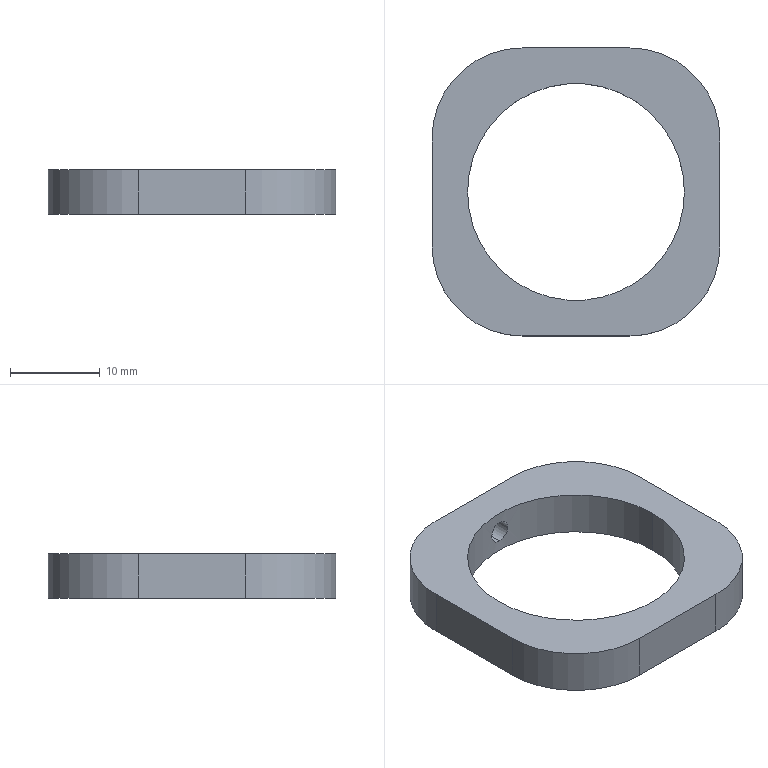Part | STEP file | QA-FC03 | 1 solid | 14 faces | box 32 x 32 x 5 mm | volume 2390 mm3 | cylinder 8 | plane 6 | commonest cylinder face diameters 20 x4 2.5 x2 24.1 x2
STEP:
#1=CARTESIAN_POINT('',(0.,0.,0.));
#2=DIRECTION('',(0.,0.,1.));
#3=DIRECTION('',(1.,0.,0.));
#4=AXIS2_PLACEMENT_3D('',#1,#2,#3);
#5=CARTESIAN_POINT('',(0.,12.05,3.75));
#6=VERTEX_POINT('',#5);
#7=CARTESIAN_POINT('',(0.,16.,3.75));
#8=VERTEX_POINT('',#7);
#9=CARTESIAN_POINT('',(0.,16.,3.75));
#10=DIRECTION('',(0.,1.,0.));
#11=VECTOR('',#10,1.);
#12=LINE('',#9,#11);
#13=CARTESIAN_POINT('',(0.,16.,2.5));
#14=DIRECTION('',(0.,1.,0.));
#15=DIRECTION('',(0.,0.,1.));
#16=AXIS2_PLACEMENT_3D('',#13,#14,#15);
#17=CYLINDRICAL_SURFACE('',#16,1.25);
#18=CARTESIAN_POINT('',(6.283,0.));
#19=DIRECTION('',(0.,1.));
#20=VECTOR('',#19,1.);
#21=LINE('',#18,#20);
#22=(GEOMETRIC_REPRESENTATION_CONTEXT(2)PARAMETRIC_REPRESENTATION_CONTEXT()REPRESENTATION_CONTEXT('',''));
#23=DEFINITIONAL_REPRESENTATION('',(#21),#22);
#24=PCURVE('',#17,#23);
#25=CARTESIAN_POINT('',(0.,16.,2.5));
#26=DIRECTION('',(0.,1.,0.));
#27=DIRECTION('',(0.,0.,1.));
#28=AXIS2_PLACEMENT_3D('',#25,#26,#27);
#29=CYLINDRICAL_SURFACE('',#28,1.25);
#30=CARTESIAN_POINT('',(0.,0.));
#31=DIRECTION('',(0.,1.));
#32=VECTOR('',#31,1.);
#33=LINE('',#30,#32);
#34=(GEOMETRIC_REPRESENTATION_CONTEXT(2)PARAMETRIC_REPRESENTATION_CONTEXT()REPRESENTATION_CONTEXT('',''));
#35=DEFINITIONAL_REPRESENTATION('',(#33),#34);
#36=PCURVE('',#29,#35);
#37=SURFACE_CURVE('',#12,(#24,#36),.PCURVE_S1.);
#38=EDGE_CURVE('',#6,#8,#37,.T.);
#39=ORIENTED_EDGE('',*,*,#38,.T.);
#40=CARTESIAN_POINT('',(0.,16.,1.25));
#41=VERTEX_POINT('',#40);
#42=CARTESIAN_POINT('',(0.,16.,2.5));
#43=DIRECTION('',(0.,1.,0.));
#44=DIRECTION('',(0.,0.,1.));
#45=AXIS2_PLACEMENT_3D('',#42,#43,#44);
#46=CIRCLE('',#45,1.25);
#47=CARTESIAN_POINT('',(0.,0.));
#48=DIRECTION('',(1.,0.));
#49=VECTOR('',#48,1.);
#50=LINE('',#47,#49);
#51=(GEOMETRIC_REPRESENTATION_CONTEXT(2)PARAMETRIC_REPRESENTATION_CONTEXT()REPRESENTATION_CONTEXT('',''));
#52=DEFINITIONAL_REPRESENTATION('',(#50),#51);
#53=PCURVE('',#17,#52);
#54=CARTESIAN_POINT('',(-16.,16.,5.));
#55=DIRECTION('',(0.,-1.,0.));
#56=DIRECTION('',(0.,0.,-1.));
#57=AXIS2_PLACEMENT_3D('',#54,#55,#56);
#58=PLANE('',#57);
#59=CARTESIAN_POINT('',(1.25,16.));
#60=CARTESIAN_POINT('',(1.25,18.165));
#61=CARTESIAN_POINT('',(3.125,17.083));
#62=CARTESIAN_POINT('',(5.,16.));
#63=CARTESIAN_POINT('',(3.125,14.917));
#64=CARTESIAN_POINT('',(1.25,13.835));
#65=CARTESIAN_POINT('',(1.25,16.));
#66=(BOUNDED_CURVE()B_SPLINE_CURVE(2,(#59,#60,#61,#62,#63,#64,#65),.UNSPECIFIED.,.T.,.F.)B_SPLINE_CURVE_WITH_KNOTS((1,2,2,2,2,1),(-2.094,0.,2.094,4.189,6.283,8.378),.UNSPECIFIED.)CURVE()GEOMETRIC_REPRESENTATION_ITEM()RATIONAL_B_SPLINE_CURVE((1.,0.5,1.,0.5,1.,0.5,1.))REPRESENTATION_ITEM(''));
#67=(GEOMETRIC_REPRESENTATION_CONTEXT(2)PARAMETRIC_REPRESENTATION_CONTEXT()REPRESENTATION_CONTEXT('',''));
#68=DEFINITIONAL_REPRESENTATION('',(#66),#67);
#69=PCURVE('',#58,#68);
#70=SURFACE_CURVE('',#46,(#53,#69),.PCURVE_S1.);
#71=EDGE_CURVE('',#41,#8,#70,.T.);
#72=ORIENTED_EDGE('',*,*,#71,.F.);
#73=CARTESIAN_POINT('',(0.,12.05,1.25));
#74=VERTEX_POINT('',#73);
#75=CARTESIAN_POINT('',(0.,16.,1.25));
#76=DIRECTION('',(0.,1.,0.));
#77=VECTOR('',#76,1.);
#78=LINE('',#75,#77);
#79=CARTESIAN_POINT('',(3.142,0.));
#80=DIRECTION('',(0.,1.));
#81=VECTOR('',#80,1.);
#82=LINE('',#79,#81);
#83=(GEOMETRIC_REPRESENTATION_CONTEXT(2)PARAMETRIC_REPRESENTATION_CONTEXT()REPRESENTATION_CONTEXT('',''));
#84=DEFINITIONAL_REPRESENTATION('',(#82),#83);
#85=PCURVE('',#17,#84);
#86=CARTESIAN_POINT('',(3.142,0.));
#87=DIRECTION('',(0.,1.));
#88=VECTOR('',#87,1.);
#89=LINE('',#86,#88);
#90=(GEOMETRIC_REPRESENTATION_CONTEXT(2)PARAMETRIC_REPRESENTATION_CONTEXT()REPRESENTATION_CONTEXT('',''));
#91=DEFINITIONAL_REPRESENTATION('',(#89),#90);
#92=PCURVE('',#29,#91);
#93=SURFACE_CURVE('',#78,(#85,#92),.PCURVE_S1.);
#94=EDGE_CURVE('',#74,#41,#93,.T.);
#95=ORIENTED_EDGE('',*,*,#94,.F.);
#96=CARTESIAN_POINT('',(0.,12.05,3.75));
#97=CARTESIAN_POINT('',(-0.1653,12.05,3.75));
#98=CARTESIAN_POINT('',(-0.3275,12.047,3.717));
#99=CARTESIAN_POINT('',(-0.6302,12.034,3.592));
#100=CARTESIAN_POINT('',(-0.7688,12.026,3.499));
#101=CARTESIAN_POINT('',(-0.9993,12.009,3.268));
#102=CARTESIAN_POINT('',(-1.092,12.001,3.129));
#103=CARTESIAN_POINT('',(-1.217,11.989,2.828));
#104=CARTESIAN_POINT('',(-1.25,11.985,2.664));
#105=CARTESIAN_POINT('',(-1.25,11.985,2.337));
#106=CARTESIAN_POINT('',(-1.218,11.988,2.173));
#107=CARTESIAN_POINT('',(-1.092,12.001,1.871));
#108=CARTESIAN_POINT('',(-1.001,12.009,1.733));
#109=CARTESIAN_POINT('',(-0.7673,12.026,1.5));
#110=CARTESIAN_POINT('',(-0.6298,12.034,1.408));
#111=CARTESIAN_POINT('',(-0.4027,12.044,1.314));
#112=CARTESIAN_POINT('',(-0.3248,12.046,1.29));
#113=CARTESIAN_POINT('',(-0.1645,12.049,1.258));
#114=CARTESIAN_POINT('',(-0.08161,12.05,1.25));
#115=CARTESIAN_POINT('',(0.,12.05,1.25));
#116=B_SPLINE_CURVE_WITH_KNOTS('',3,(#96,#97,#98,#99,#100,#101,#102,#103,#104,#105,#106,#107,#108,#109,#110,#111,#112,#113,#114,#115),.UNSPECIFIED.,.F.,.F.,(4,2,2,2,2,2,2,2,2,4),(0.,0.0004888,0.0009777,0.001467,0.001955,0.002444,0.002933,0.003422,0.003666,0.003911),.UNSPECIFIED.);
#117=CARTESIAN_POINT('',(6.283,-3.95));
#118=CARTESIAN_POINT('',(6.259,-3.95));
#119=CARTESIAN_POINT('',(6.211,-3.95));
#120=CARTESIAN_POINT('',(6.14,-3.951));
#121=CARTESIAN_POINT('',(6.068,-3.953));
#122=CARTESIAN_POINT('',(5.997,-3.955));
#123=CARTESIAN_POINT('',(5.926,-3.958));
#124=CARTESIAN_POINT('',(5.854,-3.961));
#125=CARTESIAN_POINT('',(5.783,-3.965));
#126=CARTESIAN_POINT('',(5.711,-3.969));
#127=CARTESIAN_POINT('',(5.64,-3.973));
#128=CARTESIAN_POINT('',(5.569,-3.978));
#129=CARTESIAN_POINT('',(5.498,-3.982));
#130=CARTESIAN_POINT('',(5.426,-3.987));
#131=CARTESIAN_POINT('',(5.355,-3.992));
#132=CARTESIAN_POINT('',(5.284,-3.996));
#133=CARTESIAN_POINT('',(5.212,-4.));
#134=CARTESIAN_POINT('',(5.141,-4.004));
#135=CARTESIAN_POINT('',(5.07,-4.007));
#136=CARTESIAN_POINT('',(4.999,-4.01));
#137=CARTESIAN_POINT('',(4.927,-4.012));
#138=CARTESIAN_POINT('',(4.856,-4.014));
#139=CARTESIAN_POINT('',(4.784,-4.015));
#140=CARTESIAN_POINT('',(4.713,-4.015));
#141=CARTESIAN_POINT('',(4.642,-4.015));
#142=CARTESIAN_POINT('',(4.57,-4.014));
#143=CARTESIAN_POINT('',(4.499,-4.012));
#144=CARTESIAN_POINT('',(4.427,-4.01));
#145=CARTESIAN_POINT('',(4.356,-4.007));
#146=CARTESIAN_POINT('',(4.284,-4.004));
#147=CARTESIAN_POINT('',(4.213,-4.));
#148=CARTESIAN_POINT('',(4.142,-3.996));
#149=CARTESIAN_POINT('',(4.07,-3.992));
#150=CARTESIAN_POINT('',(3.999,-3.987));
#151=CARTESIAN_POINT('',(3.927,-3.982));
#152=CARTESIAN_POINT('',(3.855,-3.978));
#153=CARTESIAN_POINT('',(3.784,-3.973));
#154=CARTESIAN_POINT('',(3.713,-3.969));
#155=CARTESIAN_POINT('',(3.641,-3.965));
#156=CARTESIAN_POINT('',(3.57,-3.961));
#157=CARTESIAN_POINT('',(3.499,-3.958));
#158=CARTESIAN_POINT('',(3.428,-3.955));
#159=CARTESIAN_POINT('',(3.356,-3.953));
#160=CARTESIAN_POINT('',(3.285,-3.951));
#161=CARTESIAN_POINT('',(3.213,-3.95));
#162=CARTESIAN_POINT('',(3.165,-3.95));
#163=CARTESIAN_POINT('',(3.142,-3.95));
#164=B_SPLINE_CURVE_WITH_KNOTS('',3,(#117,#118,#119,#120,#121,#122,#123,#124,#125,#126,#127,#128,#129,#130,#131,#132,#133,#134,#135,#136,#137,#138,#139,#140,#141,#142,#143,#144,#145,#146,#147,#148,#149,#150,#151,#152,#153,#154,#155,#156,#157,#158,#159,#160,#161,#162,#163),.UNSPECIFIED.,.F.,.F.,(4,1,1,1,1,1,1,1,1,1,1,1,1,1,1,1,1,1,1,1,1,1,1,1,1,1,1,1,1,1,1,1,1,1,1,1,1,1,1,1,1,1,1,1,4),(0.,0.00008888,0.0001778,0.0002666,0.0003555,0.0004444,0.0005333,0.0006222,0.000711,0.0007999,0.0008888,0.0009777,0.001067,0.001155,0.001244,0.001333,0.001422,0.001511,0.0016,0.001689,0.001778,0.001866,0.001955,0.002044,0.002133,0.002222,0.002311,0.0024,0.002489,0.002578,0.002666,0.002755,0.002844,0.002933,0.003022,0.003111,0.0032,0.003289,0.003377,0.003466,0.003555,0.003644,0.003733,0.003822,0.003911),.QUASI_UNIFORM_KNOTS.);
#165=(GEOMETRIC_REPRESENTATION_CONTEXT(2)PARAMETRIC_REPRESENTATION_CONTEXT()REPRESENTATION_CONTEXT('',''));
#166=DEFINITIONAL_REPRESENTATION('',(#164),#165);
#167=PCURVE('',#17,#166);
#168=CARTESIAN_POINT('',(0.,0.,5.));
#169=DIRECTION('',(0.,0.,-1.));
#170=DIRECTION('',(-1.,0.,0.));
#171=AXIS2_PLACEMENT_3D('',#168,#169,#170);
#172=CYLINDRICAL_SURFACE('',#171,12.05);
#173=CARTESIAN_POINT('',(1.571,1.25));
#174=CARTESIAN_POINT('',(1.568,1.25));
#175=CARTESIAN_POINT('',(1.563,1.252));
#176=CARTESIAN_POINT('',(1.556,1.262));
#177=CARTESIAN_POINT('',(1.549,1.278));
#178=CARTESIAN_POINT('',(1.541,1.3));
#179=CARTESIAN_POINT('',(1.534,1.328));
#180=CARTESIAN_POINT('',(1.528,1.362));
#181=CARTESIAN_POINT('',(1.521,1.402));
#182=CARTESIAN_POINT('',(1.515,1.448));
#183=CARTESIAN_POINT('',(1.508,1.499));
#184=CARTESIAN_POINT('',(1.503,1.555));
#185=CARTESIAN_POINT('',(1.497,1.616));
#186=CARTESIAN_POINT('',(1.492,1.681));
#187=CARTESIAN_POINT('',(1.488,1.75));
#188=CARTESIAN_POINT('',(1.483,1.824));
#189=CARTESIAN_POINT('',(1.48,1.901));
#190=CARTESIAN_POINT('',(1.476,1.98));
#191=CARTESIAN_POINT('',(1.473,2.062));
#192=CARTESIAN_POINT('',(1.471,2.147));
#193=CARTESIAN_POINT('',(1.469,2.234));
#194=CARTESIAN_POINT('',(1.468,2.322));
#195=CARTESIAN_POINT('',(1.467,2.41));
#196=CARTESIAN_POINT('',(1.467,2.5));
#197=CARTESIAN_POINT('',(1.467,2.589));
#198=CARTESIAN_POINT('',(1.468,2.677));
#199=CARTESIAN_POINT('',(1.469,2.765));
#200=CARTESIAN_POINT('',(1.471,2.852));
#201=CARTESIAN_POINT('',(1.473,2.937));
#202=CARTESIAN_POINT('',(1.476,3.019));
#203=CARTESIAN_POINT('',(1.48,3.099));
#204=CARTESIAN_POINT('',(1.483,3.176));
#205=CARTESIAN_POINT('',(1.488,3.249));
#206=CARTESIAN_POINT('',(1.492,3.319));
#207=CARTESIAN_POINT('',(1.497,3.385));
#208=CARTESIAN_POINT('',(1.503,3.446));
#209=CARTESIAN_POINT('',(1.509,3.502));
#210=CARTESIAN_POINT('',(1.515,3.553));
#211=CARTESIAN_POINT('',(1.521,3.598));
#212=CARTESIAN_POINT('',(1.528,3.638));
#213=CARTESIAN_POINT('',(1.535,3.672));
#214=CARTESIAN_POINT('',(1.542,3.7));
#215=CARTESIAN_POINT('',(1.549,3.722));
#216=CARTESIAN_POINT('',(1.556,3.738));
#217=CARTESIAN_POINT('',(1.563,3.748));
#218=CARTESIAN_POINT('',(1.568,3.75));
#219=CARTESIAN_POINT('',(1.571,3.75));
#220=B_SPLINE_CURVE_WITH_KNOTS('',3,(#173,#174,#175,#176,#177,#178,#179,#180,#181,#182,#183,#184,#185,#186,#187,#188,#189,#190,#191,#192,#193,#194,#195,#196,#197,#198,#199,#200,#201,#202,#203,#204,#205,#206,#207,#208,#209,#210,#211,#212,#213,#214,#215,#216,#217,#218,#219),.UNSPECIFIED.,.F.,.F.,(4,1,1,1,1,1,1,1,1,1,1,1,1,1,1,1,1,1,1,1,1,1,1,1,1,1,1,1,1,1,1,1,1,1,1,1,1,1,1,1,1,1,1,1,4),(0.,0.00008888,0.0001778,0.0002666,0.0003555,0.0004444,0.0005333,0.0006222,0.000711,0.0007999,0.0008888,0.0009777,0.001067,0.001155,0.001244,0.001333,0.001422,0.001511,0.0016,0.001689,0.001778,0.001866,0.001955,0.002044,0.002133,0.002222,0.002311,0.0024,0.002489,0.002578,0.002666,0.002755,0.002844,0.002933,0.003022,0.003111,0.0032,0.003289,0.003377,0.003466,0.003555,0.003644,0.003733,0.003822,0.003911),.QUASI_UNIFORM_KNOTS.);
#221=(GEOMETRIC_REPRESENTATION_CONTEXT(2)PARAMETRIC_REPRESENTATION_CONTEXT()REPRESENTATION_CONTEXT('',''));
#222=DEFINITIONAL_REPRESENTATION('',(#220),#221);
#223=PCURVE('',#172,#222);
#224=SURFACE_CURVE('',#116,(#167,#223),.PCURVE_S1.);
#225=EDGE_CURVE('',#6,#74,#224,.T.);
#226=ORIENTED_EDGE('',*,*,#225,.F.);
#227=EDGE_LOOP('',(#39,#72,#95,#226));
#228=FACE_BOUND('',#227,.F.);
#229=ADVANCED_FACE('',(#228),#17,.F.);
#230=CARTESIAN_POINT('',(-12.05,0.,5.));
#231=VERTEX_POINT('',#230);
#232=CARTESIAN_POINT('',(-12.05,0.,0.));
#233=VERTEX_POINT('',#232);
#234=CARTESIAN_POINT('',(-12.05,0.,5.));
#235=DIRECTION('',(0.,0.,-1.));
#236=VECTOR('',#235,1.);
#237=LINE('',#234,#236);
#238=CARTESIAN_POINT('',(0.,0.,5.));
#239=DIRECTION('',(0.,0.,-1.));
#240=DIRECTION('',(-1.,0.,0.));
#241=AXIS2_PLACEMENT_3D('',#238,#239,#240);
#242=CYLINDRICAL_SURFACE('',#241,12.05);
#243=CARTESIAN_POINT('',(6.283,0.));
#244=DIRECTION('',(0.,1.));
#245=VECTOR('',#244,1.);
#246=LINE('',#243,#245);
#247=(GEOMETRIC_REPRESENTATION_CONTEXT(2)PARAMETRIC_REPRESENTATION_CONTEXT()REPRESENTATION_CONTEXT('',''));
#248=DEFINITIONAL_REPRESENTATION('',(#246),#247);
#249=PCURVE('',#242,#248);
#250=CARTESIAN_POINT('',(0.,0.));
#251=DIRECTION('',(0.,1.));
#252=VECTOR('',#251,1.);
#253=LINE('',#250,#252);
#254=(GEOMETRIC_REPRESENTATION_CONTEXT(2)PARAMETRIC_REPRESENTATION_CONTEXT()REPRESENTATION_CONTEXT('',''));
#255=DEFINITIONAL_REPRESENTATION('',(#253),#254);
#256=PCURVE('',#172,#255);
#257=SURFACE_CURVE('',#237,(#249,#256),.PCURVE_S1.);
#258=EDGE_CURVE('',#231,#233,#257,.T.);
#259=ORIENTED_EDGE('',*,*,#258,.T.);
#260=CARTESIAN_POINT('',(12.05,0.,0.));
#261=VERTEX_POINT('',#260);
#262=CARTESIAN_POINT('',(0.,0.,0.));
#263=DIRECTION('',(0.,0.,1.));
#264=DIRECTION('',(1.,0.,0.));
#265=AXIS2_PLACEMENT_3D('',#262,#263,#264);
#266=CIRCLE('',#265,12.05);
#267=CARTESIAN_POINT('',(9.425,5.));
#268=DIRECTION('',(-1.,0.));
#269=VECTOR('',#268,1.);
#270=LINE('',#267,#269);
#271=(GEOMETRIC_REPRESENTATION_CONTEXT(2)PARAMETRIC_REPRESENTATION_CONTEXT()REPRESENTATION_CONTEXT('',''));
#272=DEFINITIONAL_REPRESENTATION('',(#270),#271);
#273=PCURVE('',#242,#272);
#274=CARTESIAN_POINT('',(0.,0.,0.));
#275=DIRECTION('',(0.,0.,-1.));
#276=DIRECTION('',(-1.,0.,0.));
#277=AXIS2_PLACEMENT_3D('',#274,#275,#276);
#278=PLANE('',#277);
#279=CARTESIAN_POINT('',(-12.05,0.));
#280=CARTESIAN_POINT('',(-12.05,20.871));
#281=CARTESIAN_POINT('',(6.025,10.436));
#282=CARTESIAN_POINT('',(24.1,0.));
#283=CARTESIAN_POINT('',(6.025,-10.436));
#284=CARTESIAN_POINT('',(-12.05,-20.871));
#285=CARTESIAN_POINT('',(-12.05,0.));
#286=(BOUNDED_CURVE()B_SPLINE_CURVE(2,(#279,#280,#281,#282,#283,#284,#285),.UNSPECIFIED.,.T.,.F.)B_SPLINE_CURVE_WITH_KNOTS((1,2,2,2,2,1),(-2.094,0.,2.094,4.189,6.283,8.378),.UNSPECIFIED.)CURVE()GEOMETRIC_REPRESENTATION_ITEM()RATIONAL_B_SPLINE_CURVE((1.,0.5,1.,0.5,1.,0.5,1.))REPRESENTATION_ITEM(''));
#287=(GEOMETRIC_REPRESENTATION_CONTEXT(2)PARAMETRIC_REPRESENTATION_CONTEXT()REPRESENTATION_CONTEXT('',''));
#288=DEFINITIONAL_REPRESENTATION('',(#286),#287);
#289=PCURVE('',#278,#288);
#290=SURFACE_CURVE('',#266,(#273,#289),.PCURVE_S1.);
#291=EDGE_CURVE('',#233,#261,#290,.T.);
#292=ORIENTED_EDGE('',*,*,#291,.T.);
#293=CARTESIAN_POINT('',(12.05,0.,5.));
#294=VERTEX_POINT('',#293);
#295=CARTESIAN_POINT('',(12.05,0.,5.));
#296=DIRECTION('',(0.,0.,-1.));
#297=VECTOR('',#296,1.);
#298=LINE('',#295,#297);
#299=CARTESIAN_POINT('',(3.142,0.));
#300=DIRECTION('',(0.,1.));
#301=VECTOR('',#300,1.);
#302=LINE('',#299,#301);
#303=(GEOMETRIC_REPRESENTATION_CONTEXT(2)PARAMETRIC_REPRESENTATION_CONTEXT()REPRESENTATION_CONTEXT('',''));
#304=DEFINITIONAL_REPRESENTATION('',(#302),#303);
#305=PCURVE('',#242,#304);
#306=CARTESIAN_POINT('',(3.142,0.));
#307=DIRECTION('',(0.,1.));
#308=VECTOR('',#307,1.);
#309=LINE('',#306,#308);
#310=(GEOMETRIC_REPRESENTATION_CONTEXT(2)PARAMETRIC_REPRESENTATION_CONTEXT()REPRESENTATION_CONTEXT('',''));
#311=DEFINITIONAL_REPRESENTATION('',(#309),#310);
#312=PCURVE('',#172,#311);
#313=SURFACE_CURVE('',#298,(#305,#312),.PCURVE_S1.);
#314=EDGE_CURVE('',#294,#261,#313,.T.);
#315=ORIENTED_EDGE('',*,*,#314,.F.);
#316=CARTESIAN_POINT('',(0.,0.,5.));
#317=DIRECTION('',(0.,0.,1.));
#318=DIRECTION('',(1.,0.,0.));
#319=AXIS2_PLACEMENT_3D('',#316,#317,#318);
#320=CIRCLE('',#319,12.05);
#321=CARTESIAN_POINT('',(9.425,0.));
#322=DIRECTION('',(-1.,0.));
#323=VECTOR('',#322,1.);
#324=LINE('',#321,#323);
#325=(GEOMETRIC_REPRESENTATION_CONTEXT(2)PARAMETRIC_REPRESENTATION_CONTEXT()REPRESENTATION_CONTEXT('',''));
#326=DEFINITIONAL_REPRESENTATION('',(#324),#325);
#327=PCURVE('',#242,#326);
#328=CARTESIAN_POINT('',(0.,0.,5.));
#329=DIRECTION('',(0.,0.,-1.));
#330=DIRECTION('',(-1.,0.,0.));
#331=AXIS2_PLACEMENT_3D('',#328,#329,#330);
#332=PLANE('',#331);
#333=CARTESIAN_POINT('',(-12.05,0.));
#334=CARTESIAN_POINT('',(-12.05,20.871));
#335=CARTESIAN_POINT('',(6.025,10.436));
#336=CARTESIAN_POINT('',(24.1,0.));
#337=CARTESIAN_POINT('',(6.025,-10.436));
#338=CARTESIAN_POINT('',(-12.05,-20.871));
#339=CARTESIAN_POINT('',(-12.05,0.));
#340=(BOUNDED_CURVE()B_SPLINE_CURVE(2,(#333,#334,#335,#336,#337,#338,#339),.UNSPECIFIED.,.T.,.F.)B_SPLINE_CURVE_WITH_KNOTS((1,2,2,2,2,1),(-2.094,0.,2.094,4.189,6.283,8.378),.UNSPECIFIED.)CURVE()GEOMETRIC_REPRESENTATION_ITEM()RATIONAL_B_SPLINE_CURVE((1.,0.5,1.,0.5,1.,0.5,1.))REPRESENTATION_ITEM(''));
#341=(GEOMETRIC_REPRESENTATION_CONTEXT(2)PARAMETRIC_REPRESENTATION_CONTEXT()REPRESENTATION_CONTEXT('',''));
#342=DEFINITIONAL_REPRESENTATION('',(#340),#341);
#343=PCURVE('',#332,#342);
#344=SURFACE_CURVE('',#320,(#327,#343),.PCURVE_S1.);
#345=EDGE_CURVE('',#231,#294,#344,.T.);
#346=ORIENTED_EDGE('',*,*,#345,.F.);
#347=EDGE_LOOP('',(#259,#292,#315,#346));
#348=FACE_BOUND('',#347,.F.);
#349=ADVANCED_FACE('',(#348),#242,.F.);
#350=CARTESIAN_POINT('',(-6.,-16.,5.));
#351=VERTEX_POINT('',#350);
#352=CARTESIAN_POINT('',(6.,-16.,5.));
#353=VERTEX_POINT('',#352);
#354=CARTESIAN_POINT('',(-16.,-16.,5.));
#355=DIRECTION('',(1.,0.,0.));
#356=VECTOR('',#355,1.);
#357=LINE('',#354,#356);
#358=CARTESIAN_POINT('',(16.,-16.));
#359=DIRECTION('',(-1.,0.));
#360=VECTOR('',#359,1.);
#361=LINE('',#358,#360);
#362=(GEOMETRIC_REPRESENTATION_CONTEXT(2)PARAMETRIC_REPRESENTATION_CONTEXT()REPRESENTATION_CONTEXT('',''));
#363=DEFINITIONAL_REPRESENTATION('',(#361),#362);
#364=PCURVE('',#332,#363);
#365=CARTESIAN_POINT('',(-16.,-16.,5.));
#366=DIRECTION('',(0.,1.,0.));
#367=DIRECTION('',(0.,0.,1.));
#368=AXIS2_PLACEMENT_3D('',#365,#366,#367);
#369=PLANE('',#368);
#370=CARTESIAN_POINT('',(0.,0.));
#371=DIRECTION('',(0.,1.));
#372=VECTOR('',#371,1.);
#373=LINE('',#370,#372);
#374=(GEOMETRIC_REPRESENTATION_CONTEXT(2)PARAMETRIC_REPRESENTATION_CONTEXT()REPRESENTATION_CONTEXT('',''));
#375=DEFINITIONAL_REPRESENTATION('',(#373),#374);
#376=PCURVE('',#369,#375);
#377=SURFACE_CURVE('',#357,(#364,#376),.PCURVE_S1.);
#378=EDGE_CURVE('',#351,#353,#377,.T.);
#379=ORIENTED_EDGE('',*,*,#378,.T.);
#380=CARTESIAN_POINT('',(16.,-6.,5.));
#381=VERTEX_POINT('',#380);
#382=CARTESIAN_POINT('',(6.,-6.,5.));
#383=DIRECTION('',(0.,0.,1.));
#384=DIRECTION('',(-1.,0.,0.));
#385=AXIS2_PLACEMENT_3D('',#382,#383,#384);
#386=CIRCLE('',#385,10.);
#387=CARTESIAN_POINT('',(4.,-6.));
#388=CARTESIAN_POINT('',(4.,-23.321));
#389=CARTESIAN_POINT('',(-11.,-14.66));
#390=CARTESIAN_POINT('',(-26.,-6.));
#391=CARTESIAN_POINT('',(-11.,2.66));
#392=CARTESIAN_POINT('',(4.,11.321));
#393=CARTESIAN_POINT('',(4.,-6.));
#394=(BOUNDED_CURVE()B_SPLINE_CURVE(2,(#387,#388,#389,#390,#391,#392,#393),.UNSPECIFIED.,.T.,.F.)B_SPLINE_CURVE_WITH_KNOTS((1,2,2,2,2,1),(-2.094,0.,2.094,4.189,6.283,8.378),.UNSPECIFIED.)CURVE()GEOMETRIC_REPRESENTATION_ITEM()RATIONAL_B_SPLINE_CURVE((1.,0.5,1.,0.5,1.,0.5,1.))REPRESENTATION_ITEM(''));
#395=(GEOMETRIC_REPRESENTATION_CONTEXT(2)PARAMETRIC_REPRESENTATION_CONTEXT()REPRESENTATION_CONTEXT('',''));
#396=DEFINITIONAL_REPRESENTATION('',(#394),#395);
#397=PCURVE('',#332,#396);
#398=CARTESIAN_POINT('',(6.,-6.,5.));
#399=DIRECTION('',(0.,0.,-1.));
#400=DIRECTION('',(-1.,0.,0.));
#401=AXIS2_PLACEMENT_3D('',#398,#399,#400);
#402=CYLINDRICAL_SURFACE('',#401,10.);
#403=CARTESIAN_POINT('',(6.283,0.));
#404=DIRECTION('',(-1.,0.));
#405=VECTOR('',#404,1.);
#406=LINE('',#403,#405);
#407=(GEOMETRIC_REPRESENTATION_CONTEXT(2)PARAMETRIC_REPRESENTATION_CONTEXT()REPRESENTATION_CONTEXT('',''));
#408=DEFINITIONAL_REPRESENTATION('',(#406),#407);
#409=PCURVE('',#402,#408);
#410=SURFACE_CURVE('',#386,(#397,#409),.PCURVE_S1.);
#411=EDGE_CURVE('',#353,#381,#410,.T.);
#412=ORIENTED_EDGE('',*,*,#411,.T.);
#413=CARTESIAN_POINT('',(16.,6.,5.));
#414=VERTEX_POINT('',#413);
#415=CARTESIAN_POINT('',(16.,-16.,5.));
#416=DIRECTION('',(0.,1.,0.));
#417=VECTOR('',#416,1.);
#418=LINE('',#415,#417);
#419=CARTESIAN_POINT('',(-16.,-16.));
#420=DIRECTION('',(0.,1.));
#421=VECTOR('',#420,1.);
#422=LINE('',#419,#421);
#423=(GEOMETRIC_REPRESENTATION_CONTEXT(2)PARAMETRIC_REPRESENTATION_CONTEXT()REPRESENTATION_CONTEXT('',''));
#424=DEFINITIONAL_REPRESENTATION('',(#422),#423);
#425=PCURVE('',#332,#424);
#426=CARTESIAN_POINT('',(16.,-16.,5.));
#427=DIRECTION('',(-1.,0.,0.));
#428=DIRECTION('',(0.,0.,1.));
#429=AXIS2_PLACEMENT_3D('',#426,#427,#428);
#430=PLANE('',#429);
#431=CARTESIAN_POINT('',(0.,0.));
#432=DIRECTION('',(0.,1.));
#433=VECTOR('',#432,1.);
#434=LINE('',#431,#433);
#435=(GEOMETRIC_REPRESENTATION_CONTEXT(2)PARAMETRIC_REPRESENTATION_CONTEXT()REPRESENTATION_CONTEXT('',''));
#436=DEFINITIONAL_REPRESENTATION('',(#434),#435);
#437=PCURVE('',#430,#436);
#438=SURFACE_CURVE('',#418,(#425,#437),.PCURVE_S1.);
#439=EDGE_CURVE('',#381,#414,#438,.T.);
#440=ORIENTED_EDGE('',*,*,#439,.T.);
#441=CARTESIAN_POINT('',(6.,16.,5.));
#442=VERTEX_POINT('',#441);
#443=CARTESIAN_POINT('',(6.,6.,5.));
#444=DIRECTION('',(0.,0.,1.));
#445=DIRECTION('',(-1.,0.,0.));
#446=AXIS2_PLACEMENT_3D('',#443,#444,#445);
#447=CIRCLE('',#446,10.);
#448=CARTESIAN_POINT('',(4.,6.));
#449=CARTESIAN_POINT('',(4.,-11.321));
#450=CARTESIAN_POINT('',(-11.,-2.66));
#451=CARTESIAN_POINT('',(-26.,6.));
#452=CARTESIAN_POINT('',(-11.,14.66));
#453=CARTESIAN_POINT('',(4.,23.321));
#454=CARTESIAN_POINT('',(4.,6.));
#455=(BOUNDED_CURVE()B_SPLINE_CURVE(2,(#448,#449,#450,#451,#452,#453,#454),.UNSPECIFIED.,.T.,.F.)B_SPLINE_CURVE_WITH_KNOTS((1,2,2,2,2,1),(-2.094,0.,2.094,4.189,6.283,8.378),.UNSPECIFIED.)CURVE()GEOMETRIC_REPRESENTATION_ITEM()RATIONAL_B_SPLINE_CURVE((1.,0.5,1.,0.5,1.,0.5,1.))REPRESENTATION_ITEM(''));
#456=(GEOMETRIC_REPRESENTATION_CONTEXT(2)PARAMETRIC_REPRESENTATION_CONTEXT()REPRESENTATION_CONTEXT('',''));
#457=DEFINITIONAL_REPRESENTATION('',(#455),#456);
#458=PCURVE('',#332,#457);
#459=CARTESIAN_POINT('',(6.,6.,5.));
#460=DIRECTION('',(0.,0.,-1.));
#461=DIRECTION('',(-1.,0.,0.));
#462=AXIS2_PLACEMENT_3D('',#459,#460,#461);
#463=CYLINDRICAL_SURFACE('',#462,10.);
#464=CARTESIAN_POINT('',(6.283,0.));
#465=DIRECTION('',(-1.,0.));
#466=VECTOR('',#465,1.);
#467=LINE('',#464,#466);
#468=(GEOMETRIC_REPRESENTATION_CONTEXT(2)PARAMETRIC_REPRESENTATION_CONTEXT()REPRESENTATION_CONTEXT('',''));
#469=DEFINITIONAL_REPRESENTATION('',(#467),#468);
#470=PCURVE('',#463,#469);
#471=SURFACE_CURVE('',#447,(#458,#470),.PCURVE_S1.);
#472=EDGE_CURVE('',#414,#442,#471,.T.);
#473=ORIENTED_EDGE('',*,*,#472,.T.);
#474=CARTESIAN_POINT('',(-6.,16.,5.));
#475=VERTEX_POINT('',#474);
#476=CARTESIAN_POINT('',(-16.,16.,5.));
#477=DIRECTION('',(-1.,0.,0.));
#478=VECTOR('',#477,1.);
#479=LINE('',#476,#478);
#480=CARTESIAN_POINT('',(16.,16.));
#481=DIRECTION('',(1.,0.));
#482=VECTOR('',#481,1.);
#483=LINE('',#480,#482);
#484=(GEOMETRIC_REPRESENTATION_CONTEXT(2)PARAMETRIC_REPRESENTATION_CONTEXT()REPRESENTATION_CONTEXT('',''));
#485=DEFINITIONAL_REPRESENTATION('',(#483),#484);
#486=PCURVE('',#332,#485);
#487=CARTESIAN_POINT('',(0.,0.));
#488=DIRECTION('',(0.,-1.));
#489=VECTOR('',#488,1.);
#490=LINE('',#487,#489);
#491=(GEOMETRIC_REPRESENTATION_CONTEXT(2)PARAMETRIC_REPRESENTATION_CONTEXT()REPRESENTATION_CONTEXT('',''));
#492=DEFINITIONAL_REPRESENTATION('',(#490),#491);
#493=PCURVE('',#58,#492);
#494=SURFACE_CURVE('',#479,(#486,#493),.PCURVE_S1.);
#495=EDGE_CURVE('',#442,#475,#494,.T.);
#496=ORIENTED_EDGE('',*,*,#495,.T.);
#497=CARTESIAN_POINT('',(-16.,6.,5.));
#498=VERTEX_POINT('',#497);
#499=CARTESIAN_POINT('',(-6.,6.,5.));
#500=DIRECTION('',(0.,0.,1.));
#501=DIRECTION('',(-1.,0.,0.));
#502=AXIS2_PLACEMENT_3D('',#499,#500,#501);
#503=CIRCLE('',#502,10.);
#504=CARTESIAN_POINT('',(16.,6.));
#505=CARTESIAN_POINT('',(16.,-11.321));
#506=CARTESIAN_POINT('',(1.,-2.66));
#507=CARTESIAN_POINT('',(-14.,6.));
#508=CARTESIAN_POINT('',(1.,14.66));
#509=CARTESIAN_POINT('',(16.,23.321));
#510=CARTESIAN_POINT('',(16.,6.));
#511=(BOUNDED_CURVE()B_SPLINE_CURVE(2,(#504,#505,#506,#507,#508,#509,#510),.UNSPECIFIED.,.T.,.F.)B_SPLINE_CURVE_WITH_KNOTS((1,2,2,2,2,1),(-2.094,0.,2.094,4.189,6.283,8.378),.UNSPECIFIED.)CURVE()GEOMETRIC_REPRESENTATION_ITEM()RATIONAL_B_SPLINE_CURVE((1.,0.5,1.,0.5,1.,0.5,1.))REPRESENTATION_ITEM(''));
#512=(GEOMETRIC_REPRESENTATION_CONTEXT(2)PARAMETRIC_REPRESENTATION_CONTEXT()REPRESENTATION_CONTEXT('',''));
#513=DEFINITIONAL_REPRESENTATION('',(#511),#512);
#514=PCURVE('',#332,#513);
#515=CARTESIAN_POINT('',(-6.,6.,5.));
#516=DIRECTION('',(0.,0.,-1.));
#517=DIRECTION('',(-1.,0.,0.));
#518=AXIS2_PLACEMENT_3D('',#515,#516,#517);
#519=CYLINDRICAL_SURFACE('',#518,10.);
#520=CARTESIAN_POINT('',(6.283,0.));
#521=DIRECTION('',(-1.,0.));
#522=VECTOR('',#521,1.);
#523=LINE('',#520,#522);
#524=(GEOMETRIC_REPRESENTATION_CONTEXT(2)PARAMETRIC_REPRESENTATION_CONTEXT()REPRESENTATION_CONTEXT('',''));
#525=DEFINITIONAL_REPRESENTATION('',(#523),#524);
#526=PCURVE('',#519,#525);
#527=SURFACE_CURVE('',#503,(#514,#526),.PCURVE_S1.);
#528=EDGE_CURVE('',#475,#498,#527,.T.);
#529=ORIENTED_EDGE('',*,*,#528,.T.);
#530=CARTESIAN_POINT('',(-16.,-6.,5.));
#531=VERTEX_POINT('',#530);
#532=CARTESIAN_POINT('',(-16.,-16.,5.));
#533=DIRECTION('',(0.,-1.,0.));
#534=VECTOR('',#533,1.);
#535=LINE('',#532,#534);
#536=CARTESIAN_POINT('',(16.,-16.));
#537=DIRECTION('',(0.,-1.));
#538=VECTOR('',#537,1.);
#539=LINE('',#536,#538);
#540=(GEOMETRIC_REPRESENTATION_CONTEXT(2)PARAMETRIC_REPRESENTATION_CONTEXT()REPRESENTATION_CONTEXT('',''));
#541=DEFINITIONAL_REPRESENTATION('',(#539),#540);
#542=PCURVE('',#332,#541);
#543=CARTESIAN_POINT('',(-16.,-16.,5.));
#544=DIRECTION('',(1.,0.,0.));
#545=DIRECTION('',(0.,0.,-1.));
#546=AXIS2_PLACEMENT_3D('',#543,#544,#545);
#547=PLANE('',#546);
#548=CARTESIAN_POINT('',(0.,0.));
#549=DIRECTION('',(0.,-1.));
#550=VECTOR('',#549,1.);
#551=LINE('',#548,#550);
#552=(GEOMETRIC_REPRESENTATION_CONTEXT(2)PARAMETRIC_REPRESENTATION_CONTEXT()REPRESENTATION_CONTEXT('',''));
#553=DEFINITIONAL_REPRESENTATION('',(#551),#552);
#554=PCURVE('',#547,#553);
#555=SURFACE_CURVE('',#535,(#542,#554),.PCURVE_S1.);
#556=EDGE_CURVE('',#498,#531,#555,.T.);
#557=ORIENTED_EDGE('',*,*,#556,.T.);
#558=CARTESIAN_POINT('',(-6.,-6.,5.));
#559=DIRECTION('',(0.,0.,1.));
#560=DIRECTION('',(-1.,0.,0.));
#561=AXIS2_PLACEMENT_3D('',#558,#559,#560);
#562=CIRCLE('',#561,10.);
#563=CARTESIAN_POINT('',(16.,-6.));
#564=CARTESIAN_POINT('',(16.,-23.321));
#565=CARTESIAN_POINT('',(1.,-14.66));
#566=CARTESIAN_POINT('',(-14.,-6.));
#567=CARTESIAN_POINT('',(1.,2.66));
#568=CARTESIAN_POINT('',(16.,11.321));
#569=CARTESIAN_POINT('',(16.,-6.));
#570=(BOUNDED_CURVE()B_SPLINE_CURVE(2,(#563,#564,#565,#566,#567,#568,#569),.UNSPECIFIED.,.T.,.F.)B_SPLINE_CURVE_WITH_KNOTS((1,2,2,2,2,1),(-2.094,0.,2.094,4.189,6.283,8.378),.UNSPECIFIED.)CURVE()GEOMETRIC_REPRESENTATION_ITEM()RATIONAL_B_SPLINE_CURVE((1.,0.5,1.,0.5,1.,0.5,1.))REPRESENTATION_ITEM(''));
#571=(GEOMETRIC_REPRESENTATION_CONTEXT(2)PARAMETRIC_REPRESENTATION_CONTEXT()REPRESENTATION_CONTEXT('',''));
#572=DEFINITIONAL_REPRESENTATION('',(#570),#571);
#573=PCURVE('',#332,#572);
#574=CARTESIAN_POINT('',(-6.,-6.,5.));
#575=DIRECTION('',(0.,0.,-1.));
#576=DIRECTION('',(-1.,0.,0.));
#577=AXIS2_PLACEMENT_3D('',#574,#575,#576);
#578=CYLINDRICAL_SURFACE('',#577,10.);
#579=CARTESIAN_POINT('',(6.283,0.));
#580=DIRECTION('',(-1.,0.));
#581=VECTOR('',#580,1.);
#582=LINE('',#579,#581);
#583=(GEOMETRIC_REPRESENTATION_CONTEXT(2)PARAMETRIC_REPRESENTATION_CONTEXT()REPRESENTATION_CONTEXT('',''));
#584=DEFINITIONAL_REPRESENTATION('',(#582),#583);
#585=PCURVE('',#578,#584);
#586=SURFACE_CURVE('',#562,(#573,#585),.PCURVE_S1.);
#587=EDGE_CURVE('',#531,#351,#586,.T.);
#588=ORIENTED_EDGE('',*,*,#587,.T.);
#589=EDGE_LOOP('',(#379,#412,#440,#473,#496,#529,#557,#588));
#590=FACE_BOUND('',#589,.T.);
#591=ORIENTED_EDGE('',*,*,#345,.F.);
#592=CARTESIAN_POINT('',(0.,0.,5.));
#593=DIRECTION('',(0.,0.,1.));
#594=DIRECTION('',(1.,0.,0.));
#595=AXIS2_PLACEMENT_3D('',#592,#593,#594);
#596=CIRCLE('',#595,12.05);
#597=CARTESIAN_POINT('',(-12.05,0.));
#598=CARTESIAN_POINT('',(-12.05,20.871));
#599=CARTESIAN_POINT('',(6.025,10.436));
#600=CARTESIAN_POINT('',(24.1,0.));
#601=CARTESIAN_POINT('',(6.025,-10.436));
#602=CARTESIAN_POINT('',(-12.05,-20.871));
#603=CARTESIAN_POINT('',(-12.05,0.));
#604=(BOUNDED_CURVE()B_SPLINE_CURVE(2,(#597,#598,#599,#600,#601,#602,#603),.UNSPECIFIED.,.T.,.F.)B_SPLINE_CURVE_WITH_KNOTS((1,2,2,2,2,1),(-2.094,0.,2.094,4.189,6.283,8.378),.UNSPECIFIED.)CURVE()GEOMETRIC_REPRESENTATION_ITEM()RATIONAL_B_SPLINE_CURVE((1.,0.5,1.,0.5,1.,0.5,1.))REPRESENTATION_ITEM(''));
#605=(GEOMETRIC_REPRESENTATION_CONTEXT(2)PARAMETRIC_REPRESENTATION_CONTEXT()REPRESENTATION_CONTEXT('',''));
#606=DEFINITIONAL_REPRESENTATION('',(#604),#605);
#607=PCURVE('',#332,#606);
#608=CARTESIAN_POINT('',(3.142,0.));
#609=DIRECTION('',(-1.,0.));
#610=VECTOR('',#609,1.);
#611=LINE('',#608,#610);
#612=(GEOMETRIC_REPRESENTATION_CONTEXT(2)PARAMETRIC_REPRESENTATION_CONTEXT()REPRESENTATION_CONTEXT('',''));
#613=DEFINITIONAL_REPRESENTATION('',(#611),#612);
#614=PCURVE('',#172,#613);
#615=SURFACE_CURVE('',#596,(#607,#614),.PCURVE_S1.);
#616=EDGE_CURVE('',#294,#231,#615,.T.);
#617=ORIENTED_EDGE('',*,*,#616,.F.);
#618=EDGE_LOOP('',(#591,#617));
#619=FACE_BOUND('',#618,.T.);
#620=ADVANCED_FACE('',(#590,#619),#332,.F.);
#621=CARTESIAN_POINT('',(16.,-6.,0.));
#622=VERTEX_POINT('',#621);
#623=CARTESIAN_POINT('',(16.,6.,0.));
#624=VERTEX_POINT('',#623);
#625=CARTESIAN_POINT('',(16.,-16.,0.));
#626=DIRECTION('',(0.,1.,0.));
#627=VECTOR('',#626,1.);
#628=LINE('',#625,#627);
#629=CARTESIAN_POINT('',(-16.,-16.));
#630=DIRECTION('',(0.,1.));
#631=VECTOR('',#630,1.);
#632=LINE('',#629,#631);
#633=(GEOMETRIC_REPRESENTATION_CONTEXT(2)PARAMETRIC_REPRESENTATION_CONTEXT()REPRESENTATION_CONTEXT('',''));
#634=DEFINITIONAL_REPRESENTATION('',(#632),#633);
#635=PCURVE('',#278,#634);
#636=CARTESIAN_POINT('',(-5.,0.));
#637=DIRECTION('',(0.,1.));
#638=VECTOR('',#637,1.);
#639=LINE('',#636,#638);
#640=(GEOMETRIC_REPRESENTATION_CONTEXT(2)PARAMETRIC_REPRESENTATION_CONTEXT()REPRESENTATION_CONTEXT('',''));
#641=DEFINITIONAL_REPRESENTATION('',(#639),#640);
#642=PCURVE('',#430,#641);
#643=SURFACE_CURVE('',#628,(#635,#642),.PCURVE_S1.);
#644=EDGE_CURVE('',#622,#624,#643,.T.);
#645=ORIENTED_EDGE('',*,*,#644,.F.);
#646=CARTESIAN_POINT('',(6.,-16.,0.));
#647=VERTEX_POINT('',#646);
#648=CARTESIAN_POINT('',(6.,-6.,0.));
#649=DIRECTION('',(0.,0.,-1.));
#650=DIRECTION('',(-1.,0.,0.));
#651=AXIS2_PLACEMENT_3D('',#648,#649,#650);
#652=CIRCLE('',#651,10.);
#653=CARTESIAN_POINT('',(-6.,-6.));
#654=DIRECTION('',(1.,0.));
#655=AXIS2_PLACEMENT_2D('',#653,#654);
#656=CIRCLE('',#655,10.);
#657=(GEOMETRIC_REPRESENTATION_CONTEXT(2)PARAMETRIC_REPRESENTATION_CONTEXT()REPRESENTATION_CONTEXT('',''));
#658=DEFINITIONAL_REPRESENTATION('',(#656),#657);
#659=PCURVE('',#278,#658);
#660=CARTESIAN_POINT('',(0.,5.));
#661=DIRECTION('',(1.,0.));
#662=VECTOR('',#661,1.);
#663=LINE('',#660,#662);
#664=(GEOMETRIC_REPRESENTATION_CONTEXT(2)PARAMETRIC_REPRESENTATION_CONTEXT()REPRESENTATION_CONTEXT('',''));
#665=DEFINITIONAL_REPRESENTATION('',(#663),#664);
#666=PCURVE('',#402,#665);
#667=SURFACE_CURVE('',#652,(#659,#666),.PCURVE_S1.);
#668=EDGE_CURVE('',#622,#647,#667,.T.);
#669=ORIENTED_EDGE('',*,*,#668,.T.);
#670=CARTESIAN_POINT('',(-6.,-16.,0.));
#671=VERTEX_POINT('',#670);
#672=CARTESIAN_POINT('',(-16.,-16.,0.));
#673=DIRECTION('',(1.,0.,0.));
#674=VECTOR('',#673,1.);
#675=LINE('',#672,#674);
#676=CARTESIAN_POINT('',(16.,-16.));
#677=DIRECTION('',(-1.,0.));
#678=VECTOR('',#677,1.);
#679=LINE('',#676,#678);
#680=(GEOMETRIC_REPRESENTATION_CONTEXT(2)PARAMETRIC_REPRESENTATION_CONTEXT()REPRESENTATION_CONTEXT('',''));
#681=DEFINITIONAL_REPRESENTATION('',(#679),#680);
#682=PCURVE('',#278,#681);
#683=CARTESIAN_POINT('',(-5.,0.));
#684=DIRECTION('',(0.,1.));
#685=VECTOR('',#684,1.);
#686=LINE('',#683,#685);
#687=(GEOMETRIC_REPRESENTATION_CONTEXT(2)PARAMETRIC_REPRESENTATION_CONTEXT()REPRESENTATION_CONTEXT('',''));
#688=DEFINITIONAL_REPRESENTATION('',(#686),#687);
#689=PCURVE('',#369,#688);
#690=SURFACE_CURVE('',#675,(#682,#689),.PCURVE_S1.);
#691=EDGE_CURVE('',#671,#647,#690,.T.);
#692=ORIENTED_EDGE('',*,*,#691,.F.);
#693=CARTESIAN_POINT('',(-16.,-6.,0.));
#694=VERTEX_POINT('',#693);
#695=CARTESIAN_POINT('',(-6.,-6.,0.));
#696=DIRECTION('',(0.,0.,-1.));
#697=DIRECTION('',(-1.,0.,0.));
#698=AXIS2_PLACEMENT_3D('',#695,#696,#697);
#699=CIRCLE('',#698,10.);
#700=CARTESIAN_POINT('',(6.,-6.));
#701=DIRECTION('',(1.,0.));
#702=AXIS2_PLACEMENT_2D('',#700,#701);
#703=CIRCLE('',#702,10.);
#704=(GEOMETRIC_REPRESENTATION_CONTEXT(2)PARAMETRIC_REPRESENTATION_CONTEXT()REPRESENTATION_CONTEXT('',''));
#705=DEFINITIONAL_REPRESENTATION('',(#703),#704);
#706=PCURVE('',#278,#705);
#707=CARTESIAN_POINT('',(0.,5.));
#708=DIRECTION('',(1.,0.));
#709=VECTOR('',#708,1.);
#710=LINE('',#707,#709);
#711=(GEOMETRIC_REPRESENTATION_CONTEXT(2)PARAMETRIC_REPRESENTATION_CONTEXT()REPRESENTATION_CONTEXT('',''));
#712=DEFINITIONAL_REPRESENTATION('',(#710),#711);
#713=PCURVE('',#578,#712);
#714=SURFACE_CURVE('',#699,(#706,#713),.PCURVE_S1.);
#715=EDGE_CURVE('',#671,#694,#714,.T.);
#716=ORIENTED_EDGE('',*,*,#715,.T.);
#717=CARTESIAN_POINT('',(-16.,6.,0.));
#718=VERTEX_POINT('',#717);
#719=CARTESIAN_POINT('',(-16.,-16.,0.));
#720=DIRECTION('',(0.,-1.,0.));
#721=VECTOR('',#720,1.);
#722=LINE('',#719,#721);
#723=CARTESIAN_POINT('',(16.,-16.));
#724=DIRECTION('',(0.,-1.));
#725=VECTOR('',#724,1.);
#726=LINE('',#723,#725);
#727=(GEOMETRIC_REPRESENTATION_CONTEXT(2)PARAMETRIC_REPRESENTATION_CONTEXT()REPRESENTATION_CONTEXT('',''));
#728=DEFINITIONAL_REPRESENTATION('',(#726),#727);
#729=PCURVE('',#278,#728);
#730=CARTESIAN_POINT('',(5.,0.));
#731=DIRECTION('',(0.,-1.));
#732=VECTOR('',#731,1.);
#733=LINE('',#730,#732);
#734=(GEOMETRIC_REPRESENTATION_CONTEXT(2)PARAMETRIC_REPRESENTATION_CONTEXT()REPRESENTATION_CONTEXT('',''));
#735=DEFINITIONAL_REPRESENTATION('',(#733),#734);
#736=PCURVE('',#547,#735);
#737=SURFACE_CURVE('',#722,(#729,#736),.PCURVE_S1.);
#738=EDGE_CURVE('',#718,#694,#737,.T.);
#739=ORIENTED_EDGE('',*,*,#738,.F.);
#740=CARTESIAN_POINT('',(-6.,16.,0.));
#741=VERTEX_POINT('',#740);
#742=CARTESIAN_POINT('',(-6.,6.,0.));
#743=DIRECTION('',(0.,0.,-1.));
#744=DIRECTION('',(-1.,0.,0.));
#745=AXIS2_PLACEMENT_3D('',#742,#743,#744);
#746=CIRCLE('',#745,10.);
#747=CARTESIAN_POINT('',(6.,6.));
#748=DIRECTION('',(1.,0.));
#749=AXIS2_PLACEMENT_2D('',#747,#748);
#750=CIRCLE('',#749,10.);
#751=(GEOMETRIC_REPRESENTATION_CONTEXT(2)PARAMETRIC_REPRESENTATION_CONTEXT()REPRESENTATION_CONTEXT('',''));
#752=DEFINITIONAL_REPRESENTATION('',(#750),#751);
#753=PCURVE('',#278,#752);
#754=CARTESIAN_POINT('',(0.,5.));
#755=DIRECTION('',(1.,0.));
#756=VECTOR('',#755,1.);
#757=LINE('',#754,#756);
#758=(GEOMETRIC_REPRESENTATION_CONTEXT(2)PARAMETRIC_REPRESENTATION_CONTEXT()REPRESENTATION_CONTEXT('',''));
#759=DEFINITIONAL_REPRESENTATION('',(#757),#758);
#760=PCURVE('',#519,#759);
#761=SURFACE_CURVE('',#746,(#753,#760),.PCURVE_S1.);
#762=EDGE_CURVE('',#718,#741,#761,.T.);
#763=ORIENTED_EDGE('',*,*,#762,.T.);
#764=CARTESIAN_POINT('',(6.,16.,0.));
#765=VERTEX_POINT('',#764);
#766=CARTESIAN_POINT('',(-16.,16.,0.));
#767=DIRECTION('',(-1.,0.,0.));
#768=VECTOR('',#767,1.);
#769=LINE('',#766,#768);
#770=CARTESIAN_POINT('',(16.,16.));
#771=DIRECTION('',(1.,0.));
#772=VECTOR('',#771,1.);
#773=LINE('',#770,#772);
#774=(GEOMETRIC_REPRESENTATION_CONTEXT(2)PARAMETRIC_REPRESENTATION_CONTEXT()REPRESENTATION_CONTEXT('',''));
#775=DEFINITIONAL_REPRESENTATION('',(#773),#774);
#776=PCURVE('',#278,#775);
#777=CARTESIAN_POINT('',(5.,0.));
#778=DIRECTION('',(0.,-1.));
#779=VECTOR('',#778,1.);
#780=LINE('',#777,#779);
#781=(GEOMETRIC_REPRESENTATION_CONTEXT(2)PARAMETRIC_REPRESENTATION_CONTEXT()REPRESENTATION_CONTEXT('',''));
#782=DEFINITIONAL_REPRESENTATION('',(#780),#781);
#783=PCURVE('',#58,#782);
#784=SURFACE_CURVE('',#769,(#776,#783),.PCURVE_S1.);
#785=EDGE_CURVE('',#765,#741,#784,.T.);
#786=ORIENTED_EDGE('',*,*,#785,.F.);
#787=CARTESIAN_POINT('',(6.,6.,0.));
#788=DIRECTION('',(0.,0.,-1.));
#789=DIRECTION('',(-1.,0.,0.));
#790=AXIS2_PLACEMENT_3D('',#787,#788,#789);
#791=CIRCLE('',#790,10.);
#792=CARTESIAN_POINT('',(-6.,6.));
#793=DIRECTION('',(1.,0.));
#794=AXIS2_PLACEMENT_2D('',#792,#793);
#795=CIRCLE('',#794,10.);
#796=(GEOMETRIC_REPRESENTATION_CONTEXT(2)PARAMETRIC_REPRESENTATION_CONTEXT()REPRESENTATION_CONTEXT('',''));
#797=DEFINITIONAL_REPRESENTATION('',(#795),#796);
#798=PCURVE('',#278,#797);
#799=CARTESIAN_POINT('',(0.,5.));
#800=DIRECTION('',(1.,0.));
#801=VECTOR('',#800,1.);
#802=LINE('',#799,#801);
#803=(GEOMETRIC_REPRESENTATION_CONTEXT(2)PARAMETRIC_REPRESENTATION_CONTEXT()REPRESENTATION_CONTEXT('',''));
#804=DEFINITIONAL_REPRESENTATION('',(#802),#803);
#805=PCURVE('',#463,#804);
#806=SURFACE_CURVE('',#791,(#798,#805),.PCURVE_S1.);
#807=EDGE_CURVE('',#765,#624,#806,.T.);
#808=ORIENTED_EDGE('',*,*,#807,.T.);
#809=EDGE_LOOP('',(#645,#669,#692,#716,#739,#763,#786,#808));
#810=FACE_BOUND('',#809,.T.);
#811=ORIENTED_EDGE('',*,*,#291,.T.);
#812=CARTESIAN_POINT('',(0.,0.,0.));
#813=DIRECTION('',(0.,0.,1.));
#814=DIRECTION('',(1.,0.,0.));
#815=AXIS2_PLACEMENT_3D('',#812,#813,#814);
#816=CIRCLE('',#815,12.05);
#817=CARTESIAN_POINT('',(-12.05,0.));
#818=CARTESIAN_POINT('',(-12.05,20.871));
#819=CARTESIAN_POINT('',(6.025,10.436));
#820=CARTESIAN_POINT('',(24.1,0.));
#821=CARTESIAN_POINT('',(6.025,-10.436));
#822=CARTESIAN_POINT('',(-12.05,-20.871));
#823=CARTESIAN_POINT('',(-12.05,0.));
#824=(BOUNDED_CURVE()B_SPLINE_CURVE(2,(#817,#818,#819,#820,#821,#822,#823),.UNSPECIFIED.,.T.,.F.)B_SPLINE_CURVE_WITH_KNOTS((1,2,2,2,2,1),(-2.094,0.,2.094,4.189,6.283,8.378),.UNSPECIFIED.)CURVE()GEOMETRIC_REPRESENTATION_ITEM()RATIONAL_B_SPLINE_CURVE((1.,0.5,1.,0.5,1.,0.5,1.))REPRESENTATION_ITEM(''));
#825=(GEOMETRIC_REPRESENTATION_CONTEXT(2)PARAMETRIC_REPRESENTATION_CONTEXT()REPRESENTATION_CONTEXT('',''));
#826=DEFINITIONAL_REPRESENTATION('',(#824),#825);
#827=PCURVE('',#278,#826);
#828=CARTESIAN_POINT('',(3.142,5.));
#829=DIRECTION('',(-1.,0.));
#830=VECTOR('',#829,1.);
#831=LINE('',#828,#830);
#832=(GEOMETRIC_REPRESENTATION_CONTEXT(2)PARAMETRIC_REPRESENTATION_CONTEXT()REPRESENTATION_CONTEXT('',''));
#833=DEFINITIONAL_REPRESENTATION('',(#831),#832);
#834=PCURVE('',#172,#833);
#835=SURFACE_CURVE('',#816,(#827,#834),.PCURVE_S1.);
#836=EDGE_CURVE('',#261,#233,#835,.T.);
#837=ORIENTED_EDGE('',*,*,#836,.T.);
#838=EDGE_LOOP('',(#811,#837));
#839=FACE_BOUND('',#838,.T.);
#840=ADVANCED_FACE('',(#810,#839),#278,.T.);
#841=ORIENTED_EDGE('',*,*,#439,.F.);
#842=CARTESIAN_POINT('',(16.,-6.,5.));
#843=DIRECTION('',(0.,0.,-1.));
#844=VECTOR('',#843,1.);
#845=LINE('',#842,#844);
#846=CARTESIAN_POINT('',(0.,10.));
#847=DIRECTION('',(-1.,0.));
#848=VECTOR('',#847,1.);
#849=LINE('',#846,#848);
#850=(GEOMETRIC_REPRESENTATION_CONTEXT(2)PARAMETRIC_REPRESENTATION_CONTEXT()REPRESENTATION_CONTEXT('',''));
#851=DEFINITIONAL_REPRESENTATION('',(#849),#850);
#852=PCURVE('',#430,#851);
#853=CARTESIAN_POINT('',(3.142,0.));
#854=DIRECTION('',(0.,1.));
#855=VECTOR('',#854,1.);
#856=LINE('',#853,#855);
#857=(GEOMETRIC_REPRESENTATION_CONTEXT(2)PARAMETRIC_REPRESENTATION_CONTEXT()REPRESENTATION_CONTEXT('',''));
#858=DEFINITIONAL_REPRESENTATION('',(#856),#857);
#859=PCURVE('',#402,#858);
#860=SURFACE_CURVE('',#845,(#852,#859),.PCURVE_S1.);
#861=EDGE_CURVE('',#381,#622,#860,.T.);
#862=ORIENTED_EDGE('',*,*,#861,.T.);
#863=ORIENTED_EDGE('',*,*,#644,.T.);
#864=CARTESIAN_POINT('',(16.,6.,5.));
#865=DIRECTION('',(0.,0.,1.));
#866=VECTOR('',#865,1.);
#867=LINE('',#864,#866);
#868=CARTESIAN_POINT('',(0.,22.));
#869=DIRECTION('',(1.,0.));
#870=VECTOR('',#869,1.);
#871=LINE('',#868,#870);
#872=(GEOMETRIC_REPRESENTATION_CONTEXT(2)PARAMETRIC_REPRESENTATION_CONTEXT()REPRESENTATION_CONTEXT('',''));
#873=DEFINITIONAL_REPRESENTATION('',(#871),#872);
#874=PCURVE('',#430,#873);
#875=CARTESIAN_POINT('',(3.142,0.));
#876=DIRECTION('',(0.,-1.));
#877=VECTOR('',#876,1.);
#878=LINE('',#875,#877);
#879=(GEOMETRIC_REPRESENTATION_CONTEXT(2)PARAMETRIC_REPRESENTATION_CONTEXT()REPRESENTATION_CONTEXT('',''));
#880=DEFINITIONAL_REPRESENTATION('',(#878),#879);
#881=PCURVE('',#463,#880);
#882=SURFACE_CURVE('',#867,(#874,#881),.PCURVE_S1.);
#883=EDGE_CURVE('',#624,#414,#882,.T.);
#884=ORIENTED_EDGE('',*,*,#883,.T.);
#885=EDGE_LOOP('',(#841,#862,#863,#884));
#886=FACE_BOUND('',#885,.T.);
#887=ADVANCED_FACE('',(#886),#430,.F.);
#888=CARTESIAN_POINT('',(0.,16.,2.5));
#889=DIRECTION('',(0.,1.,0.));
#890=DIRECTION('',(0.,0.,1.));
#891=AXIS2_PLACEMENT_3D('',#888,#889,#890);
#892=CIRCLE('',#891,1.25);
#893=CARTESIAN_POINT('',(1.25,16.));
#894=CARTESIAN_POINT('',(1.25,18.165));
#895=CARTESIAN_POINT('',(3.125,17.083));
#896=CARTESIAN_POINT('',(5.,16.));
#897=CARTESIAN_POINT('',(3.125,14.917));
#898=CARTESIAN_POINT('',(1.25,13.835));
#899=CARTESIAN_POINT('',(1.25,16.));
#900=(BOUNDED_CURVE()B_SPLINE_CURVE(2,(#893,#894,#895,#896,#897,#898,#899),.UNSPECIFIED.,.T.,.F.)B_SPLINE_CURVE_WITH_KNOTS((1,2,2,2,2,1),(-2.094,0.,2.094,4.189,6.283,8.378),.UNSPECIFIED.)CURVE()GEOMETRIC_REPRESENTATION_ITEM()RATIONAL_B_SPLINE_CURVE((1.,0.5,1.,0.5,1.,0.5,1.))REPRESENTATION_ITEM(''));
#901=(GEOMETRIC_REPRESENTATION_CONTEXT(2)PARAMETRIC_REPRESENTATION_CONTEXT()REPRESENTATION_CONTEXT('',''));
#902=DEFINITIONAL_REPRESENTATION('',(#900),#901);
#903=PCURVE('',#58,#902);
#904=CARTESIAN_POINT('',(0.,0.));
#905=DIRECTION('',(1.,0.));
#906=VECTOR('',#905,1.);
#907=LINE('',#904,#906);
#908=(GEOMETRIC_REPRESENTATION_CONTEXT(2)PARAMETRIC_REPRESENTATION_CONTEXT()REPRESENTATION_CONTEXT('',''));
#909=DEFINITIONAL_REPRESENTATION('',(#907),#908);
#910=PCURVE('',#29,#909);
#911=SURFACE_CURVE('',#892,(#903,#910),.PCURVE_S1.);
#912=EDGE_CURVE('',#8,#41,#911,.T.);
#913=ORIENTED_EDGE('',*,*,#912,.F.);
#914=ORIENTED_EDGE('',*,*,#71,.F.);
#915=EDGE_LOOP('',(#913,#914));
#916=FACE_BOUND('',#915,.T.);
#917=ORIENTED_EDGE('',*,*,#495,.F.);
#918=CARTESIAN_POINT('',(6.,16.,5.));
#919=DIRECTION('',(0.,0.,-1.));
#920=VECTOR('',#919,1.);
#921=LINE('',#918,#920);
#922=CARTESIAN_POINT('',(0.,22.));
#923=DIRECTION('',(1.,0.));
#924=VECTOR('',#923,1.);
#925=LINE('',#922,#924);
#926=(GEOMETRIC_REPRESENTATION_CONTEXT(2)PARAMETRIC_REPRESENTATION_CONTEXT()REPRESENTATION_CONTEXT('',''));
#927=DEFINITIONAL_REPRESENTATION('',(#925),#926);
#928=PCURVE('',#58,#927);
#929=CARTESIAN_POINT('',(1.571,0.));
#930=DIRECTION('',(0.,1.));
#931=VECTOR('',#930,1.);
#932=LINE('',#929,#931);
#933=(GEOMETRIC_REPRESENTATION_CONTEXT(2)PARAMETRIC_REPRESENTATION_CONTEXT()REPRESENTATION_CONTEXT('',''));
#934=DEFINITIONAL_REPRESENTATION('',(#932),#933);
#935=PCURVE('',#463,#934);
#936=SURFACE_CURVE('',#921,(#928,#935),.PCURVE_S1.);
#937=EDGE_CURVE('',#442,#765,#936,.T.);
#938=ORIENTED_EDGE('',*,*,#937,.T.);
#939=ORIENTED_EDGE('',*,*,#785,.T.);
#940=CARTESIAN_POINT('',(-6.,16.,5.));
#941=DIRECTION('',(0.,0.,1.));
#942=VECTOR('',#941,1.);
#943=LINE('',#940,#942);
#944=CARTESIAN_POINT('',(0.,10.));
#945=DIRECTION('',(-1.,0.));
#946=VECTOR('',#945,1.);
#947=LINE('',#944,#946);
#948=(GEOMETRIC_REPRESENTATION_CONTEXT(2)PARAMETRIC_REPRESENTATION_CONTEXT()REPRESENTATION_CONTEXT('',''));
#949=DEFINITIONAL_REPRESENTATION('',(#947),#948);
#950=PCURVE('',#58,#949);
#951=CARTESIAN_POINT('',(1.571,0.));
#952=DIRECTION('',(0.,-1.));
#953=VECTOR('',#952,1.);
#954=LINE('',#951,#953);
#955=(GEOMETRIC_REPRESENTATION_CONTEXT(2)PARAMETRIC_REPRESENTATION_CONTEXT()REPRESENTATION_CONTEXT('',''));
#956=DEFINITIONAL_REPRESENTATION('',(#954),#955);
#957=PCURVE('',#519,#956);
#958=SURFACE_CURVE('',#943,(#950,#957),.PCURVE_S1.);
#959=EDGE_CURVE('',#741,#475,#958,.T.);
#960=ORIENTED_EDGE('',*,*,#959,.T.);
#961=EDGE_LOOP('',(#917,#938,#939,#960));
#962=FACE_BOUND('',#961,.T.);
#963=ADVANCED_FACE('',(#916,#962),#58,.F.);
#964=ORIENTED_EDGE('',*,*,#738,.T.);
#965=CARTESIAN_POINT('',(-16.,-6.,5.));
#966=DIRECTION('',(0.,0.,1.));
#967=VECTOR('',#966,1.);
#968=LINE('',#965,#967);
#969=CARTESIAN_POINT('',(0.,10.));
#970=DIRECTION('',(-1.,0.));
#971=VECTOR('',#970,1.);
#972=LINE('',#969,#971);
#973=(GEOMETRIC_REPRESENTATION_CONTEXT(2)PARAMETRIC_REPRESENTATION_CONTEXT()REPRESENTATION_CONTEXT('',''));
#974=DEFINITIONAL_REPRESENTATION('',(#972),#973);
#975=PCURVE('',#547,#974);
#976=CARTESIAN_POINT('',(6.283,0.));
#977=DIRECTION('',(0.,-1.));
#978=VECTOR('',#977,1.);
#979=LINE('',#976,#978);
#980=(GEOMETRIC_REPRESENTATION_CONTEXT(2)PARAMETRIC_REPRESENTATION_CONTEXT()REPRESENTATION_CONTEXT('',''));
#981=DEFINITIONAL_REPRESENTATION('',(#979),#980);
#982=PCURVE('',#578,#981);
#983=SURFACE_CURVE('',#968,(#975,#982),.PCURVE_S1.);
#984=EDGE_CURVE('',#694,#531,#983,.T.);
#985=ORIENTED_EDGE('',*,*,#984,.T.);
#986=ORIENTED_EDGE('',*,*,#556,.F.);
#987=CARTESIAN_POINT('',(-16.,6.,5.));
#988=DIRECTION('',(0.,0.,-1.));
#989=VECTOR('',#988,1.);
#990=LINE('',#987,#989);
#991=CARTESIAN_POINT('',(0.,22.));
#992=DIRECTION('',(1.,0.));
#993=VECTOR('',#992,1.);
#994=LINE('',#991,#993);
#995=(GEOMETRIC_REPRESENTATION_CONTEXT(2)PARAMETRIC_REPRESENTATION_CONTEXT()REPRESENTATION_CONTEXT('',''));
#996=DEFINITIONAL_REPRESENTATION('',(#994),#995);
#997=PCURVE('',#547,#996);
#998=CARTESIAN_POINT('',(0.,0.));
#999=DIRECTION('',(0.,1.));
#1000=VECTOR('',#999,1.);
#1001=LINE('',#998,#1000);
#1002=(GEOMETRIC_REPRESENTATION_CONTEXT(2)PARAMETRIC_REPRESENTATION_CONTEXT()REPRESENTATION_CONTEXT('',''));
#1003=DEFINITIONAL_REPRESENTATION('',(#1001),#1002);
#1004=PCURVE('',#519,#1003);
#1005=SURFACE_CURVE('',#990,(#997,#1004),.PCURVE_S1.);
#1006=EDGE_CURVE('',#498,#718,#1005,.T.);
#1007=ORIENTED_EDGE('',*,*,#1006,.T.);
#1008=EDGE_LOOP('',(#964,#985,#986,#1007));
#1009=FACE_BOUND('',#1008,.T.);
#1010=ADVANCED_FACE('',(#1009),#547,.F.);
#1011=ORIENTED_EDGE('',*,*,#691,.T.);
#1012=CARTESIAN_POINT('',(6.,-16.,5.));
#1013=DIRECTION('',(0.,0.,1.));
#1014=VECTOR('',#1013,1.);
#1015=LINE('',#1012,#1014);
#1016=CARTESIAN_POINT('',(0.,22.));
#1017=DIRECTION('',(1.,0.));
#1018=VECTOR('',#1017,1.);
#1019=LINE('',#1016,#1018);
#1020=(GEOMETRIC_REPRESENTATION_CONTEXT(2)PARAMETRIC_REPRESENTATION_CONTEXT()REPRESENTATION_CONTEXT('',''));
#1021=DEFINITIONAL_REPRESENTATION('',(#1019),#1020);
#1022=PCURVE('',#369,#1021);
#1023=CARTESIAN_POINT('',(4.712,0.));
#1024=DIRECTION('',(0.,-1.));
#1025=VECTOR('',#1024,1.);
#1026=LINE('',#1023,#1025);
#1027=(GEOMETRIC_REPRESENTATION_CONTEXT(2)PARAMETRIC_REPRESENTATION_CONTEXT()REPRESENTATION_CONTEXT('',''));
#1028=DEFINITIONAL_REPRESENTATION('',(#1026),#1027);
#1029=PCURVE('',#402,#1028);
#1030=SURFACE_CURVE('',#1015,(#1022,#1029),.PCURVE_S1.);
#1031=EDGE_CURVE('',#647,#353,#1030,.T.);
#1032=ORIENTED_EDGE('',*,*,#1031,.T.);
#1033=ORIENTED_EDGE('',*,*,#378,.F.);
#1034=CARTESIAN_POINT('',(-6.,-16.,5.));
#1035=DIRECTION('',(0.,0.,-1.));
#1036=VECTOR('',#1035,1.);
#1037=LINE('',#1034,#1036);
#1038=CARTESIAN_POINT('',(0.,10.));
#1039=DIRECTION('',(-1.,0.));
#1040=VECTOR('',#1039,1.);
#1041=LINE('',#1038,#1040);
#1042=(GEOMETRIC_REPRESENTATION_CONTEXT(2)PARAMETRIC_REPRESENTATION_CONTEXT()REPRESENTATION_CONTEXT('',''));
#1043=DEFINITIONAL_REPRESENTATION('',(#1041),#1042);
#1044=PCURVE('',#369,#1043);
#1045=CARTESIAN_POINT('',(4.712,0.));
#1046=DIRECTION('',(0.,1.));
#1047=VECTOR('',#1046,1.);
#1048=LINE('',#1045,#1047);
#1049=(GEOMETRIC_REPRESENTATION_CONTEXT(2)PARAMETRIC_REPRESENTATION_CONTEXT()REPRESENTATION_CONTEXT('',''));
#1050=DEFINITIONAL_REPRESENTATION('',(#1048),#1049);
#1051=PCURVE('',#578,#1050);
#1052=SURFACE_CURVE('',#1037,(#1044,#1051),.PCURVE_S1.);
#1053=EDGE_CURVE('',#351,#671,#1052,.T.);
#1054=ORIENTED_EDGE('',*,*,#1053,.T.);
#1055=EDGE_LOOP('',(#1011,#1032,#1033,#1054));
#1056=FACE_BOUND('',#1055,.T.);
#1057=ADVANCED_FACE('',(#1056),#369,.F.);
#1058=ORIENTED_EDGE('',*,*,#836,.T.);
#1059=ORIENTED_EDGE('',*,*,#258,.F.);
#1060=ORIENTED_EDGE('',*,*,#616,.F.);
#1061=ORIENTED_EDGE('',*,*,#314,.T.);
#1062=EDGE_LOOP('',(#1058,#1059,#1060,#1061));
#1063=FACE_BOUND('',#1062,.F.);
#1064=CARTESIAN_POINT('',(0.,12.05,1.25));
#1065=CARTESIAN_POINT('',(0.1632,12.05,1.25));
#1066=CARTESIAN_POINT('',(0.3277,12.046,1.283));
#1067=CARTESIAN_POINT('',(0.6286,12.035,1.407));
#1068=CARTESIAN_POINT('',(0.768,12.026,1.5));
#1069=CARTESIAN_POINT('',(0.9986,12.009,1.731));
#1070=CARTESIAN_POINT('',(1.092,12.001,1.869));
#1071=CARTESIAN_POINT('',(1.217,11.989,2.172));
#1072=CARTESIAN_POINT('',(1.25,11.985,2.334));
#1073=CARTESIAN_POINT('',(1.25,11.985,2.664));
#1074=CARTESIAN_POINT('',(1.218,11.988,2.826));
#1075=CARTESIAN_POINT('',(1.092,12.001,3.129));
#1076=CARTESIAN_POINT('',(0.9997,12.009,3.268));
#1077=CARTESIAN_POINT('',(0.7693,12.026,3.499));
#1078=CARTESIAN_POINT('',(0.6301,12.034,3.592));
#1079=CARTESIAN_POINT('',(0.3294,12.046,3.717));
#1080=CARTESIAN_POINT('',(0.1653,12.05,3.75));
#1081=CARTESIAN_POINT('',(0.,12.05,3.75));
#1082=B_SPLINE_CURVE_WITH_KNOTS('',3,(#1064,#1065,#1066,#1067,#1068,#1069,#1070,#1071,#1072,#1073,#1074,#1075,#1076,#1077,#1078,#1079,#1080,#1081),.UNSPECIFIED.,.F.,.F.,(4,2,2,2,2,2,2,2,4),(0.003911,0.004399,0.004888,0.005377,0.005866,0.006354,0.006843,0.007332,0.00782),.UNSPECIFIED.);
#1083=CARTESIAN_POINT('',(1.571,3.75));
#1084=CARTESIAN_POINT('',(1.573,3.75));
#1085=CARTESIAN_POINT('',(1.578,3.748));
#1086=CARTESIAN_POINT('',(1.586,3.738));
#1087=CARTESIAN_POINT('',(1.593,3.722));
#1088=CARTESIAN_POINT('',(1.6,3.7));
#1089=CARTESIAN_POINT('',(1.607,3.672));
#1090=CARTESIAN_POINT('',(1.614,3.638));
#1091=CARTESIAN_POINT('',(1.621,3.598));
#1092=CARTESIAN_POINT('',(1.627,3.553));
#1093=CARTESIAN_POINT('',(1.633,3.502));
#1094=CARTESIAN_POINT('',(1.639,3.446));
#1095=CARTESIAN_POINT('',(1.644,3.385));
#1096=CARTESIAN_POINT('',(1.649,3.32));
#1097=CARTESIAN_POINT('',(1.654,3.251));
#1098=CARTESIAN_POINT('',(1.658,3.178));
#1099=CARTESIAN_POINT('',(1.662,3.101));
#1100=CARTESIAN_POINT('',(1.665,3.021));
#1101=CARTESIAN_POINT('',(1.668,2.938));
#1102=CARTESIAN_POINT('',(1.671,2.854));
#1103=CARTESIAN_POINT('',(1.672,2.768));
#1104=CARTESIAN_POINT('',(1.674,2.68));
#1105=CARTESIAN_POINT('',(1.675,2.591));
#1106=CARTESIAN_POINT('',(1.675,2.501));
#1107=CARTESIAN_POINT('',(1.675,2.411));
#1108=CARTESIAN_POINT('',(1.674,2.322));
#1109=CARTESIAN_POINT('',(1.672,2.234));
#1110=CARTESIAN_POINT('',(1.671,2.148));
#1111=CARTESIAN_POINT('',(1.668,2.063));
#1112=CARTESIAN_POINT('',(1.665,1.981));
#1113=CARTESIAN_POINT('',(1.662,1.901));
#1114=CARTESIAN_POINT('',(1.658,1.824));
#1115=CARTESIAN_POINT('',(1.654,1.751));
#1116=CARTESIAN_POINT('',(1.649,1.681));
#1117=CARTESIAN_POINT('',(1.644,1.616));
#1118=CARTESIAN_POINT('',(1.639,1.555));
#1119=CARTESIAN_POINT('',(1.633,1.499));
#1120=CARTESIAN_POINT('',(1.627,1.448));
#1121=CARTESIAN_POINT('',(1.621,1.403));
#1122=CARTESIAN_POINT('',(1.614,1.363));
#1123=CARTESIAN_POINT('',(1.607,1.328));
#1124=CARTESIAN_POINT('',(1.6,1.3));
#1125=CARTESIAN_POINT('',(1.593,1.278));
#1126=CARTESIAN_POINT('',(1.586,1.262));
#1127=CARTESIAN_POINT('',(1.578,1.252));
#1128=CARTESIAN_POINT('',(1.573,1.25));
#1129=CARTESIAN_POINT('',(1.571,1.25));
#1130=B_SPLINE_CURVE_WITH_KNOTS('',3,(#1083,#1084,#1085,#1086,#1087,#1088,#1089,#1090,#1091,#1092,#1093,#1094,#1095,#1096,#1097,#1098,#1099,#1100,#1101,#1102,#1103,#1104,#1105,#1106,#1107,#1108,#1109,#1110,#1111,#1112,#1113,#1114,#1115,#1116,#1117,#1118,#1119,#1120,#1121,#1122,#1123,#1124,#1125,#1126,#1127,#1128,#1129),.UNSPECIFIED.,.F.,.F.,(4,1,1,1,1,1,1,1,1,1,1,1,1,1,1,1,1,1,1,1,1,1,1,1,1,1,1,1,1,1,1,1,1,1,1,1,1,1,1,1,1,1,1,1,4),(0.003911,0.004,0.004088,0.004177,0.004266,0.004355,0.004444,0.004533,0.004622,0.00471,0.004799,0.004888,0.004977,0.005066,0.005155,0.005244,0.005332,0.005421,0.00551,0.005599,0.005688,0.005777,0.005866,0.005954,0.006043,0.006132,0.006221,0.00631,0.006399,0.006488,0.006576,0.006665,0.006754,0.006843,0.006932,0.007021,0.00711,0.007198,0.007287,0.007376,0.007465,0.007554,0.007643,0.007732,0.00782),.QUASI_UNIFORM_KNOTS.);
#1131=(GEOMETRIC_REPRESENTATION_CONTEXT(2)PARAMETRIC_REPRESENTATION_CONTEXT()REPRESENTATION_CONTEXT('',''));
#1132=DEFINITIONAL_REPRESENTATION('',(#1130),#1131);
#1133=PCURVE('',#172,#1132);
#1134=CARTESIAN_POINT('',(3.142,-3.95));
#1135=CARTESIAN_POINT('',(3.118,-3.95));
#1136=CARTESIAN_POINT('',(3.07,-3.95));
#1137=CARTESIAN_POINT('',(2.999,-3.951));
#1138=CARTESIAN_POINT('',(2.927,-3.953));
#1139=CARTESIAN_POINT('',(2.856,-3.955));
#1140=CARTESIAN_POINT('',(2.785,-3.958));
#1141=CARTESIAN_POINT('',(2.714,-3.961));
#1142=CARTESIAN_POINT('',(2.642,-3.965));
#1143=CARTESIAN_POINT('',(2.571,-3.969));
#1144=CARTESIAN_POINT('',(2.499,-3.973));
#1145=CARTESIAN_POINT('',(2.428,-3.978));
#1146=CARTESIAN_POINT('',(2.357,-3.982));
#1147=CARTESIAN_POINT('',(2.286,-3.987));
#1148=CARTESIAN_POINT('',(2.214,-3.992));
#1149=CARTESIAN_POINT('',(2.143,-3.996));
#1150=CARTESIAN_POINT('',(2.072,-4.));
#1151=CARTESIAN_POINT('',(2.,-4.004));
#1152=CARTESIAN_POINT('',(1.929,-4.007));
#1153=CARTESIAN_POINT('',(1.858,-4.01));
#1154=CARTESIAN_POINT('',(1.786,-4.012));
#1155=CARTESIAN_POINT('',(1.715,-4.014));
#1156=CARTESIAN_POINT('',(1.643,-4.015));
#1157=CARTESIAN_POINT('',(1.572,-4.015));
#1158=CARTESIAN_POINT('',(1.5,-4.015));
#1159=CARTESIAN_POINT('',(1.428,-4.014));
#1160=CARTESIAN_POINT('',(1.357,-4.012));
#1161=CARTESIAN_POINT('',(1.286,-4.01));
#1162=CARTESIAN_POINT('',(1.214,-4.007));
#1163=CARTESIAN_POINT('',(1.143,-4.004));
#1164=CARTESIAN_POINT('',(1.071,-4.));
#1165=CARTESIAN_POINT('',(0.9998,-3.996));
#1166=CARTESIAN_POINT('',(0.9285,-3.992));
#1167=CARTESIAN_POINT('',(0.8572,-3.987));
#1168=CARTESIAN_POINT('',(0.7861,-3.983));
#1169=CARTESIAN_POINT('',(0.7149,-3.978));
#1170=CARTESIAN_POINT('',(0.6435,-3.973));
#1171=CARTESIAN_POINT('',(0.5721,-3.969));
#1172=CARTESIAN_POINT('',(0.5007,-3.965));
#1173=CARTESIAN_POINT('',(0.4294,-3.961));
#1174=CARTESIAN_POINT('',(0.3584,-3.958));
#1175=CARTESIAN_POINT('',(0.2871,-3.955));
#1176=CARTESIAN_POINT('',(0.2156,-3.953));
#1177=CARTESIAN_POINT('',(0.1439,-3.951));
#1178=CARTESIAN_POINT('',(0.07206,-3.95));
#1179=CARTESIAN_POINT('',(0.02404,-3.95));
#1180=CARTESIAN_POINT('',(0.,-3.95));
#1181=B_SPLINE_CURVE_WITH_KNOTS('',3,(#1134,#1135,#1136,#1137,#1138,#1139,#1140,#1141,#1142,#1143,#1144,#1145,#1146,#1147,#1148,#1149,#1150,#1151,#1152,#1153,#1154,#1155,#1156,#1157,#1158,#1159,#1160,#1161,#1162,#1163,#1164,#1165,#1166,#1167,#1168,#1169,#1170,#1171,#1172,#1173,#1174,#1175,#1176,#1177,#1178,#1179,#1180),.UNSPECIFIED.,.F.,.F.,(4,1,1,1,1,1,1,1,1,1,1,1,1,1,1,1,1,1,1,1,1,1,1,1,1,1,1,1,1,1,1,1,1,1,1,1,1,1,1,1,1,1,1,1,4),(0.003911,0.004,0.004088,0.004177,0.004266,0.004355,0.004444,0.004533,0.004622,0.00471,0.004799,0.004888,0.004977,0.005066,0.005155,0.005244,0.005332,0.005421,0.00551,0.005599,0.005688,0.005777,0.005866,0.005954,0.006043,0.006132,0.006221,0.00631,0.006399,0.006488,0.006576,0.006665,0.006754,0.006843,0.006932,0.007021,0.00711,0.007198,0.007287,0.007376,0.007465,0.007554,0.007643,0.007732,0.00782),.QUASI_UNIFORM_KNOTS.);
#1182=(GEOMETRIC_REPRESENTATION_CONTEXT(2)PARAMETRIC_REPRESENTATION_CONTEXT()REPRESENTATION_CONTEXT('',''));
#1183=DEFINITIONAL_REPRESENTATION('',(#1181),#1182);
#1184=PCURVE('',#29,#1183);
#1185=SURFACE_CURVE('',#1082,(#1133,#1184),.PCURVE_S1.);
#1186=EDGE_CURVE('',#74,#6,#1185,.T.);
#1187=ORIENTED_EDGE('',*,*,#1186,.T.);
#1188=ORIENTED_EDGE('',*,*,#225,.T.);
#1189=EDGE_LOOP('',(#1187,#1188));
#1190=FACE_BOUND('',#1189,.F.);
#1191=ADVANCED_FACE('',(#1063,#1190),#172,.F.);
#1192=ORIENTED_EDGE('',*,*,#912,.F.);
#1193=ORIENTED_EDGE('',*,*,#38,.F.);
#1194=ORIENTED_EDGE('',*,*,#1186,.F.);
#1195=ORIENTED_EDGE('',*,*,#94,.T.);
#1196=EDGE_LOOP('',(#1192,#1193,#1194,#1195));
#1197=FACE_BOUND('',#1196,.F.);
#1198=ADVANCED_FACE('',(#1197),#29,.F.);
#1199=ORIENTED_EDGE('',*,*,#411,.F.);
#1200=ORIENTED_EDGE('',*,*,#1031,.F.);
#1201=ORIENTED_EDGE('',*,*,#668,.F.);
#1202=ORIENTED_EDGE('',*,*,#861,.F.);
#1203=EDGE_LOOP('',(#1199,#1200,#1201,#1202));
#1204=FACE_BOUND('',#1203,.T.);
#1205=ADVANCED_FACE('',(#1204),#402,.T.);
#1206=ORIENTED_EDGE('',*,*,#587,.F.);
#1207=ORIENTED_EDGE('',*,*,#984,.F.);
#1208=ORIENTED_EDGE('',*,*,#715,.F.);
#1209=ORIENTED_EDGE('',*,*,#1053,.F.);
#1210=EDGE_LOOP('',(#1206,#1207,#1208,#1209));
#1211=FACE_BOUND('',#1210,.T.);
#1212=ADVANCED_FACE('',(#1211),#578,.T.);
#1213=ORIENTED_EDGE('',*,*,#472,.F.);
#1214=ORIENTED_EDGE('',*,*,#883,.F.);
#1215=ORIENTED_EDGE('',*,*,#807,.F.);
#1216=ORIENTED_EDGE('',*,*,#937,.F.);
#1217=EDGE_LOOP('',(#1213,#1214,#1215,#1216));
#1218=FACE_BOUND('',#1217,.T.);
#1219=ADVANCED_FACE('',(#1218),#463,.T.);
#1220=ORIENTED_EDGE('',*,*,#528,.F.);
#1221=ORIENTED_EDGE('',*,*,#959,.F.);
#1222=ORIENTED_EDGE('',*,*,#762,.F.);
#1223=ORIENTED_EDGE('',*,*,#1006,.F.);
#1224=EDGE_LOOP('',(#1220,#1221,#1222,#1223));
#1225=FACE_BOUND('',#1224,.T.);
#1226=ADVANCED_FACE('',(#1225),#519,.T.);
#1227=CLOSED_SHELL('',(#229,#349,#620,#840,#887,#963,#1010,#1057,#1191,#1198,#1205,#1212,#1219,#1226));
#1228=MANIFOLD_SOLID_BREP('',#1227);
#1229=(LENGTH_UNIT()NAMED_UNIT(*)SI_UNIT(.MILLI.,.METRE.));
#1230=UNCERTAINTY_MEASURE_WITH_UNIT(LENGTH_MEASURE(0.00001),#1229,'','');
#1231=(NAMED_UNIT(*)PLANE_ANGLE_UNIT()SI_UNIT($,.RADIAN.));
#1232=(NAMED_UNIT(*)SI_UNIT($,.STERADIAN.)SOLID_ANGLE_UNIT());
#1233=(GEOMETRIC_REPRESENTATION_CONTEXT(3)GLOBAL_UNCERTAINTY_ASSIGNED_CONTEXT((#1230))GLOBAL_UNIT_ASSIGNED_CONTEXT((#1229,#1231,#1232))REPRESENTATION_CONTEXT('',''));
#1234=ADVANCED_BREP_SHAPE_REPRESENTATION('',(#4,#1228),#1233);